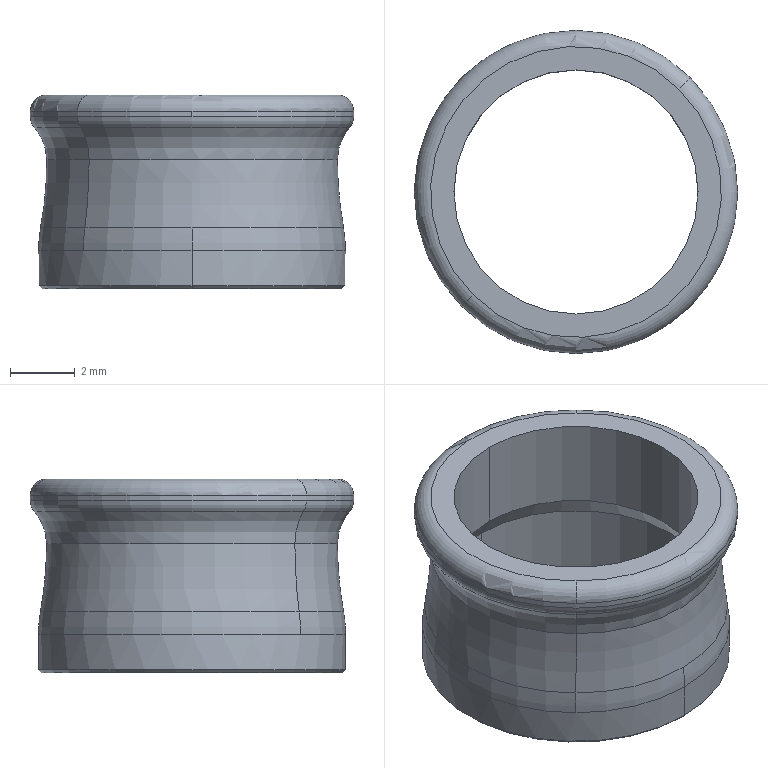Part | STEP file | ASND-0110-4216111500 | 1 solid | 26 faces | box 10 x 10 x 6 mm | volume 119.565 mm3 | torus 8 | cylinder 8 | other 4 | cone 4 | plane 2 | commonest cylinder face diameters 7.55 x2 8.3 x2 9.5 x2 10 x2